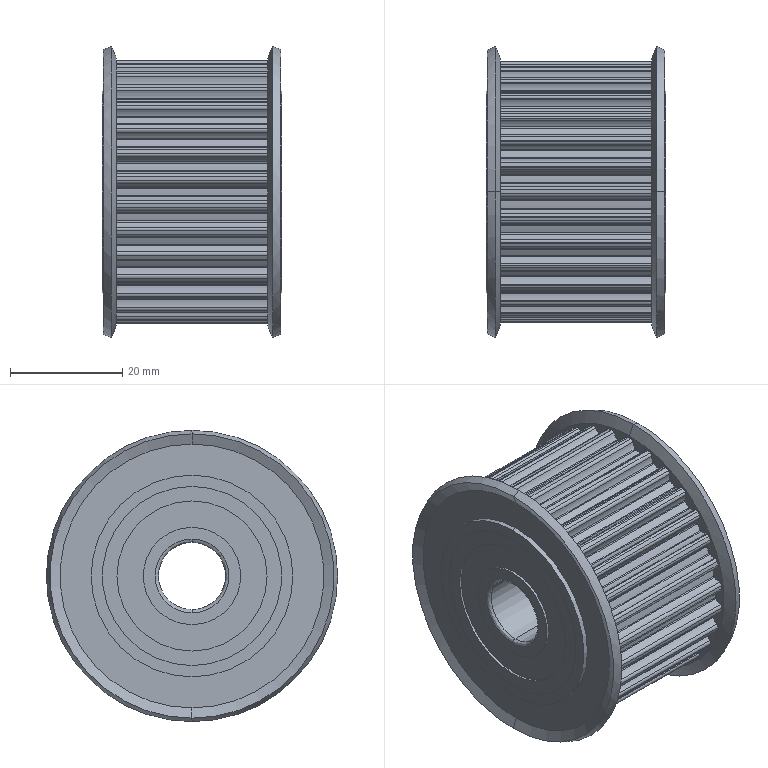Part | SolidWorks | features BaseBody 3 | 3 solids | 343 faces | box 32 x 52 x 52 mm | volume 41430 mm3 | cylinder 299 | plane 20 | cone 12 | spline 12 | commonest cylinder face diameters 1.1 x72 0.5 x68 6.55 x64 46.79 x31 43.25 x30 17.4 x8